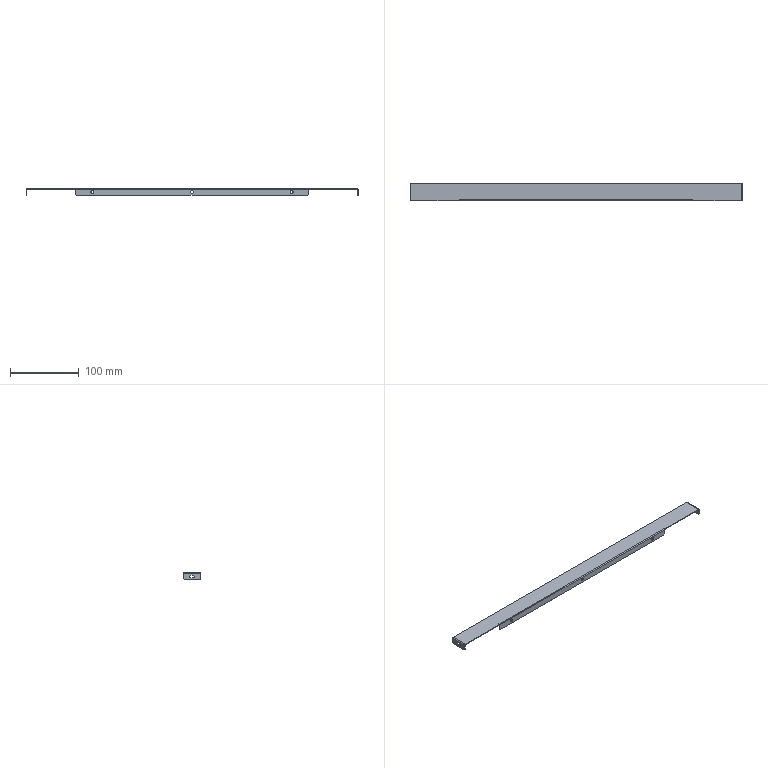Part | STEP file | 1 solid | 58 faces | box 483 x 25 x 10 mm | volume 15373 mm3 | plane 42 | cylinder 16 | commonest cylinder face diameters 4 x6 3.5 x4 0.4 x3 2.4 x3